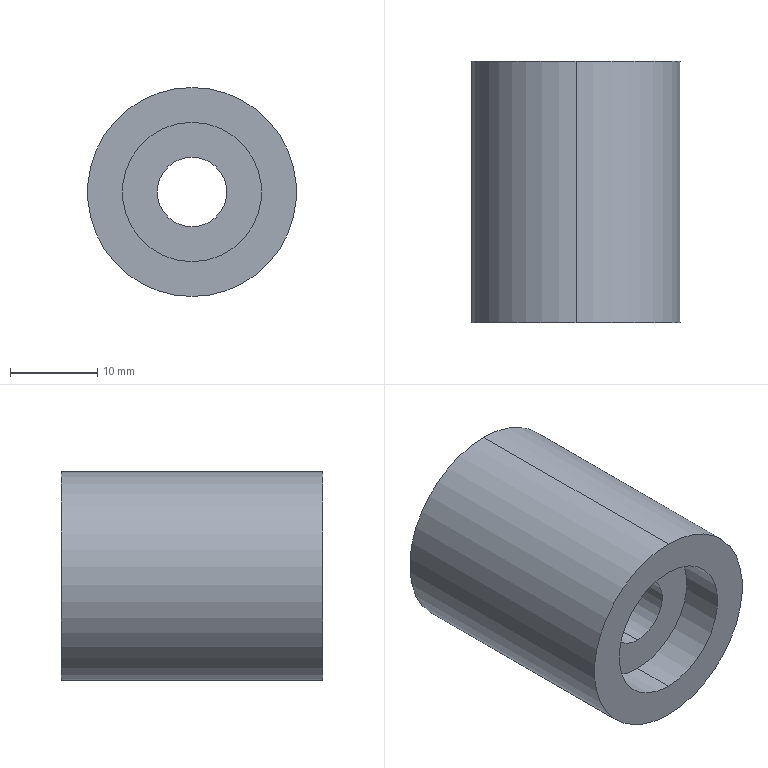Part | STEP file | Polisher small pulley | 1 solid | 12 faces | box 24 x 30 x 24 mm | volume 10556 mm3 | cylinder 8 | plane 4 | commonest cylinder face diameters 16 x4 8 x2 24 x2
STEP:
#1=CARTESIAN_POINT('',(0.,0.,0.));
#2=DIRECTION('',(0.,0.,1.));
#3=DIRECTION('',(1.,0.,0.));
#4=AXIS2_PLACEMENT_3D('',#1,#2,#3);
#5=CARTESIAN_POINT('',(0.,-10.,-8.));
#6=VERTEX_POINT('',#5);
#7=CARTESIAN_POINT('',(0.,-15.,-8.));
#8=VERTEX_POINT('',#7);
#9=CARTESIAN_POINT('',(0.,-10.,-8.));
#10=DIRECTION('',(0.,-1.,0.));
#11=VECTOR('',#10,1.);
#12=LINE('',#9,#11);
#13=CARTESIAN_POINT('',(0.,-10.,0.));
#14=DIRECTION('',(0.,-1.,0.));
#15=DIRECTION('',(0.,0.,-1.));
#16=AXIS2_PLACEMENT_3D('',#13,#14,#15);
#17=CYLINDRICAL_SURFACE('',#16,8.);
#18=CARTESIAN_POINT('',(6.283,0.));
#19=DIRECTION('',(0.,1.));
#20=VECTOR('',#19,1.);
#21=LINE('',#18,#20);
#22=(GEOMETRIC_REPRESENTATION_CONTEXT(2)PARAMETRIC_REPRESENTATION_CONTEXT()REPRESENTATION_CONTEXT('',''));
#23=DEFINITIONAL_REPRESENTATION('',(#21),#22);
#24=PCURVE('',#17,#23);
#25=CARTESIAN_POINT('',(0.,-10.,0.));
#26=DIRECTION('',(0.,-1.,0.));
#27=DIRECTION('',(0.,0.,-1.));
#28=AXIS2_PLACEMENT_3D('',#25,#26,#27);
#29=CYLINDRICAL_SURFACE('',#28,8.);
#30=CARTESIAN_POINT('',(0.,0.));
#31=DIRECTION('',(0.,1.));
#32=VECTOR('',#31,1.);
#33=LINE('',#30,#32);
#34=(GEOMETRIC_REPRESENTATION_CONTEXT(2)PARAMETRIC_REPRESENTATION_CONTEXT()REPRESENTATION_CONTEXT('',''));
#35=DEFINITIONAL_REPRESENTATION('',(#33),#34);
#36=PCURVE('',#29,#35);
#37=SURFACE_CURVE('',#12,(#24,#36),.PCURVE_S1.);
#38=EDGE_CURVE('',#6,#8,#37,.T.);
#39=ORIENTED_EDGE('',*,*,#38,.T.);
#40=CARTESIAN_POINT('',(0.,-15.,8.));
#41=VERTEX_POINT('',#40);
#42=CARTESIAN_POINT('',(0.,-15.,0.));
#43=DIRECTION('',(0.,-1.,0.));
#44=DIRECTION('',(0.,0.,-1.));
#45=AXIS2_PLACEMENT_3D('',#42,#43,#44);
#46=CIRCLE('',#45,8.);
#47=CARTESIAN_POINT('',(0.,5.));
#48=DIRECTION('',(1.,0.));
#49=VECTOR('',#48,1.);
#50=LINE('',#47,#49);
#51=(GEOMETRIC_REPRESENTATION_CONTEXT(2)PARAMETRIC_REPRESENTATION_CONTEXT()REPRESENTATION_CONTEXT('',''));
#52=DEFINITIONAL_REPRESENTATION('',(#50),#51);
#53=PCURVE('',#17,#52);
#54=CARTESIAN_POINT('',(0.,-15.,0.));
#55=DIRECTION('',(0.,1.,0.));
#56=DIRECTION('',(0.,0.,1.));
#57=AXIS2_PLACEMENT_3D('',#54,#55,#56);
#58=PLANE('',#57);
#59=CARTESIAN_POINT('',(-8.,0.));
#60=CARTESIAN_POINT('',(-8.,13.856));
#61=CARTESIAN_POINT('',(4.,6.928));
#62=CARTESIAN_POINT('',(16.,0.));
#63=CARTESIAN_POINT('',(4.,-6.928));
#64=CARTESIAN_POINT('',(-8.,-13.856));
#65=CARTESIAN_POINT('',(-8.,0.));
#66=(BOUNDED_CURVE()B_SPLINE_CURVE(2,(#59,#60,#61,#62,#63,#64,#65),.UNSPECIFIED.,.T.,.F.)B_SPLINE_CURVE_WITH_KNOTS((1,2,2,2,2,1),(-2.094,0.,2.094,4.189,6.283,8.378),.UNSPECIFIED.)CURVE()GEOMETRIC_REPRESENTATION_ITEM()RATIONAL_B_SPLINE_CURVE((1.,0.5,1.,0.5,1.,0.5,1.))REPRESENTATION_ITEM(''));
#67=(GEOMETRIC_REPRESENTATION_CONTEXT(2)PARAMETRIC_REPRESENTATION_CONTEXT()REPRESENTATION_CONTEXT('',''));
#68=DEFINITIONAL_REPRESENTATION('',(#66),#67);
#69=PCURVE('',#58,#68);
#70=SURFACE_CURVE('',#46,(#53,#69),.PCURVE_S1.);
#71=EDGE_CURVE('',#41,#8,#70,.T.);
#72=ORIENTED_EDGE('',*,*,#71,.F.);
#73=CARTESIAN_POINT('',(0.,-10.,8.));
#74=VERTEX_POINT('',#73);
#75=CARTESIAN_POINT('',(0.,-10.,8.));
#76=DIRECTION('',(0.,-1.,0.));
#77=VECTOR('',#76,1.);
#78=LINE('',#75,#77);
#79=CARTESIAN_POINT('',(3.142,0.));
#80=DIRECTION('',(0.,1.));
#81=VECTOR('',#80,1.);
#82=LINE('',#79,#81);
#83=(GEOMETRIC_REPRESENTATION_CONTEXT(2)PARAMETRIC_REPRESENTATION_CONTEXT()REPRESENTATION_CONTEXT('',''));
#84=DEFINITIONAL_REPRESENTATION('',(#82),#83);
#85=PCURVE('',#17,#84);
#86=CARTESIAN_POINT('',(3.142,0.));
#87=DIRECTION('',(0.,1.));
#88=VECTOR('',#87,1.);
#89=LINE('',#86,#88);
#90=(GEOMETRIC_REPRESENTATION_CONTEXT(2)PARAMETRIC_REPRESENTATION_CONTEXT()REPRESENTATION_CONTEXT('',''));
#91=DEFINITIONAL_REPRESENTATION('',(#89),#90);
#92=PCURVE('',#29,#91);
#93=SURFACE_CURVE('',#78,(#85,#92),.PCURVE_S1.);
#94=EDGE_CURVE('',#74,#41,#93,.T.);
#95=ORIENTED_EDGE('',*,*,#94,.F.);
#96=CARTESIAN_POINT('',(0.,-10.,0.));
#97=DIRECTION('',(0.,-1.,0.));
#98=DIRECTION('',(0.,0.,-1.));
#99=AXIS2_PLACEMENT_3D('',#96,#97,#98);
#100=CIRCLE('',#99,8.);
#101=CARTESIAN_POINT('',(0.,0.));
#102=DIRECTION('',(1.,0.));
#103=VECTOR('',#102,1.);
#104=LINE('',#101,#103);
#105=(GEOMETRIC_REPRESENTATION_CONTEXT(2)PARAMETRIC_REPRESENTATION_CONTEXT()REPRESENTATION_CONTEXT('',''));
#106=DEFINITIONAL_REPRESENTATION('',(#104),#105);
#107=PCURVE('',#17,#106);
#108=CARTESIAN_POINT('',(0.,-10.,0.));
#109=DIRECTION('',(0.,-1.,0.));
#110=DIRECTION('',(0.,0.,-1.));
#111=AXIS2_PLACEMENT_3D('',#108,#109,#110);
#112=PLANE('',#111);
#113=CARTESIAN_POINT('',(0.,0.));
#114=DIRECTION('',(1.,0.));
#115=AXIS2_PLACEMENT_2D('',#113,#114);
#116=CIRCLE('',#115,8.);
#117=(GEOMETRIC_REPRESENTATION_CONTEXT(2)PARAMETRIC_REPRESENTATION_CONTEXT()REPRESENTATION_CONTEXT('',''));
#118=DEFINITIONAL_REPRESENTATION('',(#116),#117);
#119=PCURVE('',#112,#118);
#120=SURFACE_CURVE('',#100,(#107,#119),.PCURVE_S1.);
#121=EDGE_CURVE('',#74,#6,#120,.T.);
#122=ORIENTED_EDGE('',*,*,#121,.T.);
#123=EDGE_LOOP('',(#39,#72,#95,#122));
#124=FACE_BOUND('',#123,.F.);
#125=ADVANCED_FACE('',(#124),#17,.F.);
#126=CARTESIAN_POINT('',(0.,10.,8.));
#127=VERTEX_POINT('',#126);
#128=CARTESIAN_POINT('',(0.,15.,8.));
#129=VERTEX_POINT('',#128);
#130=CARTESIAN_POINT('',(0.,10.,8.));
#131=DIRECTION('',(0.,1.,0.));
#132=VECTOR('',#131,1.);
#133=LINE('',#130,#132);
#134=CARTESIAN_POINT('',(0.,10.,0.));
#135=DIRECTION('',(0.,1.,0.));
#136=DIRECTION('',(0.,0.,1.));
#137=AXIS2_PLACEMENT_3D('',#134,#135,#136);
#138=CYLINDRICAL_SURFACE('',#137,8.);
#139=CARTESIAN_POINT('',(6.283,0.));
#140=DIRECTION('',(0.,1.));
#141=VECTOR('',#140,1.);
#142=LINE('',#139,#141);
#143=(GEOMETRIC_REPRESENTATION_CONTEXT(2)PARAMETRIC_REPRESENTATION_CONTEXT()REPRESENTATION_CONTEXT('',''));
#144=DEFINITIONAL_REPRESENTATION('',(#142),#143);
#145=PCURVE('',#138,#144);
#146=CARTESIAN_POINT('',(0.,10.,0.));
#147=DIRECTION('',(0.,1.,0.));
#148=DIRECTION('',(0.,0.,1.));
#149=AXIS2_PLACEMENT_3D('',#146,#147,#148);
#150=CYLINDRICAL_SURFACE('',#149,8.);
#151=CARTESIAN_POINT('',(0.,0.));
#152=DIRECTION('',(0.,1.));
#153=VECTOR('',#152,1.);
#154=LINE('',#151,#153);
#155=(GEOMETRIC_REPRESENTATION_CONTEXT(2)PARAMETRIC_REPRESENTATION_CONTEXT()REPRESENTATION_CONTEXT('',''));
#156=DEFINITIONAL_REPRESENTATION('',(#154),#155);
#157=PCURVE('',#150,#156);
#158=SURFACE_CURVE('',#133,(#145,#157),.PCURVE_S1.);
#159=EDGE_CURVE('',#127,#129,#158,.T.);
#160=ORIENTED_EDGE('',*,*,#159,.T.);
#161=CARTESIAN_POINT('',(0.,15.,-8.));
#162=VERTEX_POINT('',#161);
#163=CARTESIAN_POINT('',(0.,15.,0.));
#164=DIRECTION('',(0.,1.,0.));
#165=DIRECTION('',(0.,0.,1.));
#166=AXIS2_PLACEMENT_3D('',#163,#164,#165);
#167=CIRCLE('',#166,8.);
#168=CARTESIAN_POINT('',(0.,5.));
#169=DIRECTION('',(1.,0.));
#170=VECTOR('',#169,1.);
#171=LINE('',#168,#170);
#172=(GEOMETRIC_REPRESENTATION_CONTEXT(2)PARAMETRIC_REPRESENTATION_CONTEXT()REPRESENTATION_CONTEXT('',''));
#173=DEFINITIONAL_REPRESENTATION('',(#171),#172);
#174=PCURVE('',#138,#173);
#175=CARTESIAN_POINT('',(0.,15.,0.));
#176=DIRECTION('',(0.,1.,0.));
#177=DIRECTION('',(0.,0.,1.));
#178=AXIS2_PLACEMENT_3D('',#175,#176,#177);
#179=PLANE('',#178);
#180=CARTESIAN_POINT('',(0.,0.));
#181=DIRECTION('',(1.,0.));
#182=AXIS2_PLACEMENT_2D('',#180,#181);
#183=CIRCLE('',#182,8.);
#184=(GEOMETRIC_REPRESENTATION_CONTEXT(2)PARAMETRIC_REPRESENTATION_CONTEXT()REPRESENTATION_CONTEXT('',''));
#185=DEFINITIONAL_REPRESENTATION('',(#183),#184);
#186=PCURVE('',#179,#185);
#187=SURFACE_CURVE('',#167,(#174,#186),.PCURVE_S1.);
#188=EDGE_CURVE('',#162,#129,#187,.T.);
#189=ORIENTED_EDGE('',*,*,#188,.F.);
#190=CARTESIAN_POINT('',(0.,10.,-8.));
#191=VERTEX_POINT('',#190);
#192=CARTESIAN_POINT('',(0.,10.,-8.));
#193=DIRECTION('',(0.,1.,0.));
#194=VECTOR('',#193,1.);
#195=LINE('',#192,#194);
#196=CARTESIAN_POINT('',(3.142,0.));
#197=DIRECTION('',(0.,1.));
#198=VECTOR('',#197,1.);
#199=LINE('',#196,#198);
#200=(GEOMETRIC_REPRESENTATION_CONTEXT(2)PARAMETRIC_REPRESENTATION_CONTEXT()REPRESENTATION_CONTEXT('',''));
#201=DEFINITIONAL_REPRESENTATION('',(#199),#200);
#202=PCURVE('',#138,#201);
#203=CARTESIAN_POINT('',(3.142,0.));
#204=DIRECTION('',(0.,1.));
#205=VECTOR('',#204,1.);
#206=LINE('',#203,#205);
#207=(GEOMETRIC_REPRESENTATION_CONTEXT(2)PARAMETRIC_REPRESENTATION_CONTEXT()REPRESENTATION_CONTEXT('',''));
#208=DEFINITIONAL_REPRESENTATION('',(#206),#207);
#209=PCURVE('',#150,#208);
#210=SURFACE_CURVE('',#195,(#202,#209),.PCURVE_S1.);
#211=EDGE_CURVE('',#191,#162,#210,.T.);
#212=ORIENTED_EDGE('',*,*,#211,.F.);
#213=CARTESIAN_POINT('',(0.,10.,0.));
#214=DIRECTION('',(0.,1.,0.));
#215=DIRECTION('',(0.,0.,1.));
#216=AXIS2_PLACEMENT_3D('',#213,#214,#215);
#217=CIRCLE('',#216,8.);
#218=CARTESIAN_POINT('',(0.,0.));
#219=DIRECTION('',(1.,0.));
#220=VECTOR('',#219,1.);
#221=LINE('',#218,#220);
#222=(GEOMETRIC_REPRESENTATION_CONTEXT(2)PARAMETRIC_REPRESENTATION_CONTEXT()REPRESENTATION_CONTEXT('',''));
#223=DEFINITIONAL_REPRESENTATION('',(#221),#222);
#224=PCURVE('',#138,#223);
#225=CARTESIAN_POINT('',(0.,10.,0.));
#226=DIRECTION('',(0.,1.,0.));
#227=DIRECTION('',(0.,0.,1.));
#228=AXIS2_PLACEMENT_3D('',#225,#226,#227);
#229=PLANE('',#228);
#230=CARTESIAN_POINT('',(0.,0.));
#231=DIRECTION('',(1.,0.));
#232=AXIS2_PLACEMENT_2D('',#230,#231);
#233=CIRCLE('',#232,8.);
#234=(GEOMETRIC_REPRESENTATION_CONTEXT(2)PARAMETRIC_REPRESENTATION_CONTEXT()REPRESENTATION_CONTEXT('',''));
#235=DEFINITIONAL_REPRESENTATION('',(#233),#234);
#236=PCURVE('',#229,#235);
#237=SURFACE_CURVE('',#217,(#224,#236),.PCURVE_S1.);
#238=EDGE_CURVE('',#191,#127,#237,.T.);
#239=ORIENTED_EDGE('',*,*,#238,.T.);
#240=EDGE_LOOP('',(#160,#189,#212,#239));
#241=FACE_BOUND('',#240,.F.);
#242=ADVANCED_FACE('',(#241),#138,.F.);
#243=CARTESIAN_POINT('',(0.,15.,12.));
#244=VERTEX_POINT('',#243);
#245=CARTESIAN_POINT('',(0.,15.,-12.));
#246=VERTEX_POINT('',#245);
#247=CARTESIAN_POINT('',(0.,15.,0.));
#248=DIRECTION('',(0.,1.,0.));
#249=DIRECTION('',(0.,0.,1.));
#250=AXIS2_PLACEMENT_3D('',#247,#248,#249);
#251=CIRCLE('',#250,12.);
#252=CARTESIAN_POINT('',(0.,15.,0.));
#253=DIRECTION('',(0.,-1.,0.));
#254=DIRECTION('',(0.,0.,-1.));
#255=AXIS2_PLACEMENT_3D('',#252,#253,#254);
#256=CYLINDRICAL_SURFACE('',#255,12.);
#257=CARTESIAN_POINT('',(3.142,0.));
#258=DIRECTION('',(-1.,0.));
#259=VECTOR('',#258,1.);
#260=LINE('',#257,#259);
#261=(GEOMETRIC_REPRESENTATION_CONTEXT(2)PARAMETRIC_REPRESENTATION_CONTEXT()REPRESENTATION_CONTEXT('',''));
#262=DEFINITIONAL_REPRESENTATION('',(#260),#261);
#263=PCURVE('',#256,#262);
#264=CARTESIAN_POINT('',(0.,0.));
#265=DIRECTION('',(1.,0.));
#266=AXIS2_PLACEMENT_2D('',#264,#265);
#267=CIRCLE('',#266,12.);
#268=(GEOMETRIC_REPRESENTATION_CONTEXT(2)PARAMETRIC_REPRESENTATION_CONTEXT()REPRESENTATION_CONTEXT('',''));
#269=DEFINITIONAL_REPRESENTATION('',(#267),#268);
#270=PCURVE('',#179,#269);
#271=SURFACE_CURVE('',#251,(#263,#270),.PCURVE_S1.);
#272=EDGE_CURVE('',#244,#246,#271,.T.);
#273=ORIENTED_EDGE('',*,*,#272,.F.);
#274=CARTESIAN_POINT('',(0.,-15.,12.));
#275=VERTEX_POINT('',#274);
#276=CARTESIAN_POINT('',(0.,15.,12.));
#277=DIRECTION('',(0.,-1.,0.));
#278=VECTOR('',#277,1.);
#279=LINE('',#276,#278);
#280=CARTESIAN_POINT('',(3.142,0.));
#281=DIRECTION('',(0.,1.));
#282=VECTOR('',#281,1.);
#283=LINE('',#280,#282);
#284=(GEOMETRIC_REPRESENTATION_CONTEXT(2)PARAMETRIC_REPRESENTATION_CONTEXT()REPRESENTATION_CONTEXT('',''));
#285=DEFINITIONAL_REPRESENTATION('',(#283),#284);
#286=PCURVE('',#256,#285);
#287=CARTESIAN_POINT('',(0.,15.,0.));
#288=DIRECTION('',(0.,-1.,0.));
#289=DIRECTION('',(0.,0.,-1.));
#290=AXIS2_PLACEMENT_3D('',#287,#288,#289);
#291=CYLINDRICAL_SURFACE('',#290,12.);
#292=CARTESIAN_POINT('',(3.142,0.));
#293=DIRECTION('',(0.,1.));
#294=VECTOR('',#293,1.);
#295=LINE('',#292,#294);
#296=(GEOMETRIC_REPRESENTATION_CONTEXT(2)PARAMETRIC_REPRESENTATION_CONTEXT()REPRESENTATION_CONTEXT('',''));
#297=DEFINITIONAL_REPRESENTATION('',(#295),#296);
#298=PCURVE('',#291,#297);
#299=SURFACE_CURVE('',#279,(#286,#298),.PCURVE_S1.);
#300=EDGE_CURVE('',#244,#275,#299,.T.);
#301=ORIENTED_EDGE('',*,*,#300,.T.);
#302=CARTESIAN_POINT('',(0.,-15.,-12.));
#303=VERTEX_POINT('',#302);
#304=CARTESIAN_POINT('',(0.,-15.,0.));
#305=DIRECTION('',(0.,1.,0.));
#306=DIRECTION('',(0.,0.,1.));
#307=AXIS2_PLACEMENT_3D('',#304,#305,#306);
#308=CIRCLE('',#307,12.);
#309=CARTESIAN_POINT('',(3.142,30.));
#310=DIRECTION('',(-1.,0.));
#311=VECTOR('',#310,1.);
#312=LINE('',#309,#311);
#313=(GEOMETRIC_REPRESENTATION_CONTEXT(2)PARAMETRIC_REPRESENTATION_CONTEXT()REPRESENTATION_CONTEXT('',''));
#314=DEFINITIONAL_REPRESENTATION('',(#312),#313);
#315=PCURVE('',#256,#314);
#316=CARTESIAN_POINT('',(0.,0.));
#317=DIRECTION('',(1.,0.));
#318=AXIS2_PLACEMENT_2D('',#316,#317);
#319=CIRCLE('',#318,12.);
#320=(GEOMETRIC_REPRESENTATION_CONTEXT(2)PARAMETRIC_REPRESENTATION_CONTEXT()REPRESENTATION_CONTEXT('',''));
#321=DEFINITIONAL_REPRESENTATION('',(#319),#320);
#322=PCURVE('',#58,#321);
#323=SURFACE_CURVE('',#308,(#315,#322),.PCURVE_S1.);
#324=EDGE_CURVE('',#275,#303,#323,.T.);
#325=ORIENTED_EDGE('',*,*,#324,.T.);
#326=CARTESIAN_POINT('',(0.,15.,-12.));
#327=DIRECTION('',(0.,-1.,0.));
#328=VECTOR('',#327,1.);
#329=LINE('',#326,#328);
#330=CARTESIAN_POINT('',(0.,0.));
#331=DIRECTION('',(0.,1.));
#332=VECTOR('',#331,1.);
#333=LINE('',#330,#332);
#334=(GEOMETRIC_REPRESENTATION_CONTEXT(2)PARAMETRIC_REPRESENTATION_CONTEXT()REPRESENTATION_CONTEXT('',''));
#335=DEFINITIONAL_REPRESENTATION('',(#333),#334);
#336=PCURVE('',#256,#335);
#337=CARTESIAN_POINT('',(6.283,0.));
#338=DIRECTION('',(0.,1.));
#339=VECTOR('',#338,1.);
#340=LINE('',#337,#339);
#341=(GEOMETRIC_REPRESENTATION_CONTEXT(2)PARAMETRIC_REPRESENTATION_CONTEXT()REPRESENTATION_CONTEXT('',''));
#342=DEFINITIONAL_REPRESENTATION('',(#340),#341);
#343=PCURVE('',#291,#342);
#344=SURFACE_CURVE('',#329,(#336,#343),.PCURVE_S1.);
#345=EDGE_CURVE('',#246,#303,#344,.T.);
#346=ORIENTED_EDGE('',*,*,#345,.F.);
#347=EDGE_LOOP('',(#273,#301,#325,#346));
#348=FACE_BOUND('',#347,.T.);
#349=ADVANCED_FACE('',(#348),#256,.T.);
#350=CARTESIAN_POINT('',(0.,-10.,4.));
#351=VERTEX_POINT('',#350);
#352=CARTESIAN_POINT('',(0.,10.,4.));
#353=VERTEX_POINT('',#352);
#354=CARTESIAN_POINT('',(0.,-15.,4.));
#355=DIRECTION('',(0.,1.,0.));
#356=VECTOR('',#355,1.);
#357=LINE('',#354,#356);
#358=CARTESIAN_POINT('',(0.,-15.,0.));
#359=DIRECTION('',(0.,1.,0.));
#360=DIRECTION('',(0.,0.,1.));
#361=AXIS2_PLACEMENT_3D('',#358,#359,#360);
#362=CYLINDRICAL_SURFACE('',#361,4.);
#363=CARTESIAN_POINT('',(6.283,0.));
#364=DIRECTION('',(0.,1.));
#365=VECTOR('',#364,1.);
#366=LINE('',#363,#365);
#367=(GEOMETRIC_REPRESENTATION_CONTEXT(2)PARAMETRIC_REPRESENTATION_CONTEXT()REPRESENTATION_CONTEXT('',''));
#368=DEFINITIONAL_REPRESENTATION('',(#366),#367);
#369=PCURVE('',#362,#368);
#370=CARTESIAN_POINT('',(0.,-15.,0.));
#371=DIRECTION('',(0.,1.,0.));
#372=DIRECTION('',(0.,0.,1.));
#373=AXIS2_PLACEMENT_3D('',#370,#371,#372);
#374=CYLINDRICAL_SURFACE('',#373,4.);
#375=CARTESIAN_POINT('',(0.,0.));
#376=DIRECTION('',(0.,1.));
#377=VECTOR('',#376,1.);
#378=LINE('',#375,#377);
#379=(GEOMETRIC_REPRESENTATION_CONTEXT(2)PARAMETRIC_REPRESENTATION_CONTEXT()REPRESENTATION_CONTEXT('',''));
#380=DEFINITIONAL_REPRESENTATION('',(#378),#379);
#381=PCURVE('',#374,#380);
#382=SURFACE_CURVE('',#357,(#369,#381),.PCURVE_S1.);
#383=EDGE_CURVE('',#351,#353,#382,.T.);
#384=ORIENTED_EDGE('',*,*,#383,.T.);
#385=CARTESIAN_POINT('',(0.,10.,-4.));
#386=VERTEX_POINT('',#385);
#387=CARTESIAN_POINT('',(0.,10.,0.));
#388=DIRECTION('',(0.,1.,0.));
#389=DIRECTION('',(0.,0.,1.));
#390=AXIS2_PLACEMENT_3D('',#387,#388,#389);
#391=CIRCLE('',#390,4.);
#392=CARTESIAN_POINT('',(0.,25.));
#393=DIRECTION('',(1.,0.));
#394=VECTOR('',#393,1.);
#395=LINE('',#392,#394);
#396=(GEOMETRIC_REPRESENTATION_CONTEXT(2)PARAMETRIC_REPRESENTATION_CONTEXT()REPRESENTATION_CONTEXT('',''));
#397=DEFINITIONAL_REPRESENTATION('',(#395),#396);
#398=PCURVE('',#362,#397);
#399=CARTESIAN_POINT('',(0.,0.));
#400=DIRECTION('',(1.,0.));
#401=AXIS2_PLACEMENT_2D('',#399,#400);
#402=CIRCLE('',#401,4.);
#403=(GEOMETRIC_REPRESENTATION_CONTEXT(2)PARAMETRIC_REPRESENTATION_CONTEXT()REPRESENTATION_CONTEXT('',''));
#404=DEFINITIONAL_REPRESENTATION('',(#402),#403);
#405=PCURVE('',#229,#404);
#406=SURFACE_CURVE('',#391,(#398,#405),.PCURVE_S1.);
#407=EDGE_CURVE('',#386,#353,#406,.T.);
#408=ORIENTED_EDGE('',*,*,#407,.F.);
#409=CARTESIAN_POINT('',(0.,-10.,-4.));
#410=VERTEX_POINT('',#409);
#411=CARTESIAN_POINT('',(0.,-15.,-4.));
#412=DIRECTION('',(0.,1.,0.));
#413=VECTOR('',#412,1.);
#414=LINE('',#411,#413);
#415=CARTESIAN_POINT('',(3.142,0.));
#416=DIRECTION('',(0.,1.));
#417=VECTOR('',#416,1.);
#418=LINE('',#415,#417);
#419=(GEOMETRIC_REPRESENTATION_CONTEXT(2)PARAMETRIC_REPRESENTATION_CONTEXT()REPRESENTATION_CONTEXT('',''));
#420=DEFINITIONAL_REPRESENTATION('',(#418),#419);
#421=PCURVE('',#362,#420);
#422=CARTESIAN_POINT('',(3.142,0.));
#423=DIRECTION('',(0.,1.));
#424=VECTOR('',#423,1.);
#425=LINE('',#422,#424);
#426=(GEOMETRIC_REPRESENTATION_CONTEXT(2)PARAMETRIC_REPRESENTATION_CONTEXT()REPRESENTATION_CONTEXT('',''));
#427=DEFINITIONAL_REPRESENTATION('',(#425),#426);
#428=PCURVE('',#374,#427);
#429=SURFACE_CURVE('',#414,(#421,#428),.PCURVE_S1.);
#430=EDGE_CURVE('',#410,#386,#429,.T.);
#431=ORIENTED_EDGE('',*,*,#430,.F.);
#432=CARTESIAN_POINT('',(0.,-10.,0.));
#433=DIRECTION('',(0.,1.,0.));
#434=DIRECTION('',(0.,0.,-1.));
#435=AXIS2_PLACEMENT_3D('',#432,#433,#434);
#436=CIRCLE('',#435,4.);
#437=CARTESIAN_POINT('',(3.142,5.));
#438=DIRECTION('',(1.,0.));
#439=VECTOR('',#438,1.);
#440=LINE('',#437,#439);
#441=(GEOMETRIC_REPRESENTATION_CONTEXT(2)PARAMETRIC_REPRESENTATION_CONTEXT()REPRESENTATION_CONTEXT('',''));
#442=DEFINITIONAL_REPRESENTATION('',(#440),#441);
#443=PCURVE('',#362,#442);
#444=CARTESIAN_POINT('',(4.,0.));
#445=CARTESIAN_POINT('',(4.,-6.928));
#446=CARTESIAN_POINT('',(-2.,-3.464));
#447=CARTESIAN_POINT('',(-8.,0.));
#448=CARTESIAN_POINT('',(-2.,3.464));
#449=CARTESIAN_POINT('',(4.,6.928));
#450=CARTESIAN_POINT('',(4.,0.));
#451=(BOUNDED_CURVE()B_SPLINE_CURVE(2,(#444,#445,#446,#447,#448,#449,#450),.UNSPECIFIED.,.T.,.F.)B_SPLINE_CURVE_WITH_KNOTS((1,2,2,2,2,1),(-2.094,0.,2.094,4.189,6.283,8.378),.UNSPECIFIED.)CURVE()GEOMETRIC_REPRESENTATION_ITEM()RATIONAL_B_SPLINE_CURVE((1.,0.5,1.,0.5,1.,0.5,1.))REPRESENTATION_ITEM(''));
#452=(GEOMETRIC_REPRESENTATION_CONTEXT(2)PARAMETRIC_REPRESENTATION_CONTEXT()REPRESENTATION_CONTEXT('',''));
#453=DEFINITIONAL_REPRESENTATION('',(#451),#452);
#454=PCURVE('',#112,#453);
#455=SURFACE_CURVE('',#436,(#443,#454),.PCURVE_S1.);
#456=EDGE_CURVE('',#410,#351,#455,.T.);
#457=ORIENTED_EDGE('',*,*,#456,.T.);
#458=EDGE_LOOP('',(#384,#408,#431,#457));
#459=FACE_BOUND('',#458,.F.);
#460=ADVANCED_FACE('',(#459),#362,.F.);
#461=CARTESIAN_POINT('',(0.,10.,0.));
#462=DIRECTION('',(0.,1.,0.));
#463=DIRECTION('',(0.,0.,1.));
#464=AXIS2_PLACEMENT_3D('',#461,#462,#463);
#465=CIRCLE('',#464,4.);
#466=CARTESIAN_POINT('',(0.,25.));
#467=DIRECTION('',(1.,0.));
#468=VECTOR('',#467,1.);
#469=LINE('',#466,#468);
#470=(GEOMETRIC_REPRESENTATION_CONTEXT(2)PARAMETRIC_REPRESENTATION_CONTEXT()REPRESENTATION_CONTEXT('',''));
#471=DEFINITIONAL_REPRESENTATION('',(#469),#470);
#472=PCURVE('',#374,#471);
#473=CARTESIAN_POINT('',(0.,0.));
#474=DIRECTION('',(1.,0.));
#475=AXIS2_PLACEMENT_2D('',#473,#474);
#476=CIRCLE('',#475,4.);
#477=(GEOMETRIC_REPRESENTATION_CONTEXT(2)PARAMETRIC_REPRESENTATION_CONTEXT()REPRESENTATION_CONTEXT('',''));
#478=DEFINITIONAL_REPRESENTATION('',(#476),#477);
#479=PCURVE('',#229,#478);
#480=SURFACE_CURVE('',#465,(#472,#479),.PCURVE_S1.);
#481=EDGE_CURVE('',#353,#386,#480,.T.);
#482=ORIENTED_EDGE('',*,*,#481,.F.);
#483=ORIENTED_EDGE('',*,*,#383,.F.);
#484=CARTESIAN_POINT('',(0.,-10.,0.));
#485=DIRECTION('',(0.,1.,0.));
#486=DIRECTION('',(0.,0.,-1.));
#487=AXIS2_PLACEMENT_3D('',#484,#485,#486);
#488=CIRCLE('',#487,4.);
#489=CARTESIAN_POINT('',(-3.142,5.));
#490=DIRECTION('',(1.,0.));
#491=VECTOR('',#490,1.);
#492=LINE('',#489,#491);
#493=(GEOMETRIC_REPRESENTATION_CONTEXT(2)PARAMETRIC_REPRESENTATION_CONTEXT()REPRESENTATION_CONTEXT('',''));
#494=DEFINITIONAL_REPRESENTATION('',(#492),#493);
#495=PCURVE('',#374,#494);
#496=CARTESIAN_POINT('',(4.,0.));
#497=CARTESIAN_POINT('',(4.,-6.928));
#498=CARTESIAN_POINT('',(-2.,-3.464));
#499=CARTESIAN_POINT('',(-8.,0.));
#500=CARTESIAN_POINT('',(-2.,3.464));
#501=CARTESIAN_POINT('',(4.,6.928));
#502=CARTESIAN_POINT('',(4.,0.));
#503=(BOUNDED_CURVE()B_SPLINE_CURVE(2,(#496,#497,#498,#499,#500,#501,#502),.UNSPECIFIED.,.T.,.F.)B_SPLINE_CURVE_WITH_KNOTS((1,2,2,2,2,1),(-2.094,0.,2.094,4.189,6.283,8.378),.UNSPECIFIED.)CURVE()GEOMETRIC_REPRESENTATION_ITEM()RATIONAL_B_SPLINE_CURVE((1.,0.5,1.,0.5,1.,0.5,1.))REPRESENTATION_ITEM(''));
#504=(GEOMETRIC_REPRESENTATION_CONTEXT(2)PARAMETRIC_REPRESENTATION_CONTEXT()REPRESENTATION_CONTEXT('',''));
#505=DEFINITIONAL_REPRESENTATION('',(#503),#504);
#506=PCURVE('',#112,#505);
#507=SURFACE_CURVE('',#488,(#495,#506),.PCURVE_S1.);
#508=EDGE_CURVE('',#351,#410,#507,.T.);
#509=ORIENTED_EDGE('',*,*,#508,.T.);
#510=ORIENTED_EDGE('',*,*,#430,.T.);
#511=EDGE_LOOP('',(#482,#483,#509,#510));
#512=FACE_BOUND('',#511,.F.);
#513=ADVANCED_FACE('',(#512),#374,.F.);
#514=ORIENTED_EDGE('',*,*,#300,.F.);
#515=CARTESIAN_POINT('',(0.,15.,0.));
#516=DIRECTION('',(0.,1.,0.));
#517=DIRECTION('',(0.,0.,1.));
#518=AXIS2_PLACEMENT_3D('',#515,#516,#517);
#519=CIRCLE('',#518,12.);
#520=CARTESIAN_POINT('',(9.425,0.));
#521=DIRECTION('',(-1.,0.));
#522=VECTOR('',#521,1.);
#523=LINE('',#520,#522);
#524=(GEOMETRIC_REPRESENTATION_CONTEXT(2)PARAMETRIC_REPRESENTATION_CONTEXT()REPRESENTATION_CONTEXT('',''));
#525=DEFINITIONAL_REPRESENTATION('',(#523),#524);
#526=PCURVE('',#291,#525);
#527=CARTESIAN_POINT('',(0.,0.));
#528=DIRECTION('',(1.,0.));
#529=AXIS2_PLACEMENT_2D('',#527,#528);
#530=CIRCLE('',#529,12.);
#531=(GEOMETRIC_REPRESENTATION_CONTEXT(2)PARAMETRIC_REPRESENTATION_CONTEXT()REPRESENTATION_CONTEXT('',''));
#532=DEFINITIONAL_REPRESENTATION('',(#530),#531);
#533=PCURVE('',#179,#532);
#534=SURFACE_CURVE('',#519,(#526,#533),.PCURVE_S1.);
#535=EDGE_CURVE('',#246,#244,#534,.T.);
#536=ORIENTED_EDGE('',*,*,#535,.F.);
#537=ORIENTED_EDGE('',*,*,#345,.T.);
#538=CARTESIAN_POINT('',(0.,-15.,0.));
#539=DIRECTION('',(0.,1.,0.));
#540=DIRECTION('',(0.,0.,1.));
#541=AXIS2_PLACEMENT_3D('',#538,#539,#540);
#542=CIRCLE('',#541,12.);
#543=CARTESIAN_POINT('',(9.425,30.));
#544=DIRECTION('',(-1.,0.));
#545=VECTOR('',#544,1.);
#546=LINE('',#543,#545);
#547=(GEOMETRIC_REPRESENTATION_CONTEXT(2)PARAMETRIC_REPRESENTATION_CONTEXT()REPRESENTATION_CONTEXT('',''));
#548=DEFINITIONAL_REPRESENTATION('',(#546),#547);
#549=PCURVE('',#291,#548);
#550=CARTESIAN_POINT('',(0.,0.));
#551=DIRECTION('',(1.,0.));
#552=AXIS2_PLACEMENT_2D('',#550,#551);
#553=CIRCLE('',#552,12.);
#554=(GEOMETRIC_REPRESENTATION_CONTEXT(2)PARAMETRIC_REPRESENTATION_CONTEXT()REPRESENTATION_CONTEXT('',''));
#555=DEFINITIONAL_REPRESENTATION('',(#553),#554);
#556=PCURVE('',#58,#555);
#557=SURFACE_CURVE('',#542,(#549,#556),.PCURVE_S1.);
#558=EDGE_CURVE('',#303,#275,#557,.T.);
#559=ORIENTED_EDGE('',*,*,#558,.T.);
#560=EDGE_LOOP('',(#514,#536,#537,#559));
#561=FACE_BOUND('',#560,.T.);
#562=ADVANCED_FACE('',(#561),#291,.T.);
#563=CARTESIAN_POINT('',(0.,15.,0.));
#564=DIRECTION('',(0.,1.,0.));
#565=DIRECTION('',(0.,0.,1.));
#566=AXIS2_PLACEMENT_3D('',#563,#564,#565);
#567=CIRCLE('',#566,8.);
#568=CARTESIAN_POINT('',(0.,0.));
#569=DIRECTION('',(1.,0.));
#570=AXIS2_PLACEMENT_2D('',#568,#569);
#571=CIRCLE('',#570,8.);
#572=(GEOMETRIC_REPRESENTATION_CONTEXT(2)PARAMETRIC_REPRESENTATION_CONTEXT()REPRESENTATION_CONTEXT('',''));
#573=DEFINITIONAL_REPRESENTATION('',(#571),#572);
#574=PCURVE('',#179,#573);
#575=CARTESIAN_POINT('',(0.,5.));
#576=DIRECTION('',(1.,0.));
#577=VECTOR('',#576,1.);
#578=LINE('',#575,#577);
#579=(GEOMETRIC_REPRESENTATION_CONTEXT(2)PARAMETRIC_REPRESENTATION_CONTEXT()REPRESENTATION_CONTEXT('',''));
#580=DEFINITIONAL_REPRESENTATION('',(#578),#579);
#581=PCURVE('',#150,#580);
#582=SURFACE_CURVE('',#567,(#574,#581),.PCURVE_S1.);
#583=EDGE_CURVE('',#129,#162,#582,.T.);
#584=ORIENTED_EDGE('',*,*,#583,.F.);
#585=ORIENTED_EDGE('',*,*,#188,.F.);
#586=EDGE_LOOP('',(#584,#585));
#587=FACE_BOUND('',#586,.T.);
#588=ORIENTED_EDGE('',*,*,#535,.T.);
#589=ORIENTED_EDGE('',*,*,#272,.T.);
#590=EDGE_LOOP('',(#588,#589));
#591=FACE_BOUND('',#590,.T.);
#592=ADVANCED_FACE('',(#587,#591),#179,.T.);
#593=CARTESIAN_POINT('',(0.,-15.,0.));
#594=DIRECTION('',(0.,-1.,0.));
#595=DIRECTION('',(0.,0.,-1.));
#596=AXIS2_PLACEMENT_3D('',#593,#594,#595);
#597=CIRCLE('',#596,8.);
#598=CARTESIAN_POINT('',(-8.,0.));
#599=CARTESIAN_POINT('',(-8.,13.856));
#600=CARTESIAN_POINT('',(4.,6.928));
#601=CARTESIAN_POINT('',(16.,0.));
#602=CARTESIAN_POINT('',(4.,-6.928));
#603=CARTESIAN_POINT('',(-8.,-13.856));
#604=CARTESIAN_POINT('',(-8.,0.));
#605=(BOUNDED_CURVE()B_SPLINE_CURVE(2,(#598,#599,#600,#601,#602,#603,#604),.UNSPECIFIED.,.T.,.F.)B_SPLINE_CURVE_WITH_KNOTS((1,2,2,2,2,1),(-2.094,0.,2.094,4.189,6.283,8.378),.UNSPECIFIED.)CURVE()GEOMETRIC_REPRESENTATION_ITEM()RATIONAL_B_SPLINE_CURVE((1.,0.5,1.,0.5,1.,0.5,1.))REPRESENTATION_ITEM(''));
#606=(GEOMETRIC_REPRESENTATION_CONTEXT(2)PARAMETRIC_REPRESENTATION_CONTEXT()REPRESENTATION_CONTEXT('',''));
#607=DEFINITIONAL_REPRESENTATION('',(#605),#606);
#608=PCURVE('',#58,#607);
#609=CARTESIAN_POINT('',(0.,5.));
#610=DIRECTION('',(1.,0.));
#611=VECTOR('',#610,1.);
#612=LINE('',#609,#611);
#613=(GEOMETRIC_REPRESENTATION_CONTEXT(2)PARAMETRIC_REPRESENTATION_CONTEXT()REPRESENTATION_CONTEXT('',''));
#614=DEFINITIONAL_REPRESENTATION('',(#612),#613);
#615=PCURVE('',#29,#614);
#616=SURFACE_CURVE('',#597,(#608,#615),.PCURVE_S1.);
#617=EDGE_CURVE('',#8,#41,#616,.T.);
#618=ORIENTED_EDGE('',*,*,#617,.F.);
#619=ORIENTED_EDGE('',*,*,#71,.F.);
#620=EDGE_LOOP('',(#618,#619));
#621=FACE_BOUND('',#620,.T.);
#622=ORIENTED_EDGE('',*,*,#558,.F.);
#623=ORIENTED_EDGE('',*,*,#324,.F.);
#624=EDGE_LOOP('',(#622,#623));
#625=FACE_BOUND('',#624,.T.);
#626=ADVANCED_FACE('',(#621,#625),#58,.F.);
#627=ORIENTED_EDGE('',*,*,#583,.F.);
#628=ORIENTED_EDGE('',*,*,#159,.F.);
#629=CARTESIAN_POINT('',(0.,10.,0.));
#630=DIRECTION('',(0.,1.,0.));
#631=DIRECTION('',(0.,0.,1.));
#632=AXIS2_PLACEMENT_3D('',#629,#630,#631);
#633=CIRCLE('',#632,8.);
#634=CARTESIAN_POINT('',(0.,0.));
#635=DIRECTION('',(1.,0.));
#636=VECTOR('',#635,1.);
#637=LINE('',#634,#636);
#638=(GEOMETRIC_REPRESENTATION_CONTEXT(2)PARAMETRIC_REPRESENTATION_CONTEXT()REPRESENTATION_CONTEXT('',''));
#639=DEFINITIONAL_REPRESENTATION('',(#637),#638);
#640=PCURVE('',#150,#639);
#641=CARTESIAN_POINT('',(0.,0.));
#642=DIRECTION('',(1.,0.));
#643=AXIS2_PLACEMENT_2D('',#641,#642);
#644=CIRCLE('',#643,8.);
#645=(GEOMETRIC_REPRESENTATION_CONTEXT(2)PARAMETRIC_REPRESENTATION_CONTEXT()REPRESENTATION_CONTEXT('',''));
#646=DEFINITIONAL_REPRESENTATION('',(#644),#645);
#647=PCURVE('',#229,#646);
#648=SURFACE_CURVE('',#633,(#640,#647),.PCURVE_S1.);
#649=EDGE_CURVE('',#127,#191,#648,.T.);
#650=ORIENTED_EDGE('',*,*,#649,.T.);
#651=ORIENTED_EDGE('',*,*,#211,.T.);
#652=EDGE_LOOP('',(#627,#628,#650,#651));
#653=FACE_BOUND('',#652,.F.);
#654=ADVANCED_FACE('',(#653),#150,.F.);
#655=ORIENTED_EDGE('',*,*,#481,.F.);
#656=ORIENTED_EDGE('',*,*,#407,.F.);
#657=EDGE_LOOP('',(#655,#656));
#658=FACE_BOUND('',#657,.T.);
#659=ORIENTED_EDGE('',*,*,#649,.T.);
#660=ORIENTED_EDGE('',*,*,#238,.T.);
#661=EDGE_LOOP('',(#659,#660));
#662=FACE_BOUND('',#661,.T.);
#663=ADVANCED_FACE('',(#658,#662),#229,.T.);
#664=CARTESIAN_POINT('',(0.,-10.,0.));
#665=DIRECTION('',(0.,-1.,0.));
#666=DIRECTION('',(0.,0.,-1.));
#667=AXIS2_PLACEMENT_3D('',#664,#665,#666);
#668=CIRCLE('',#667,8.);
#669=CARTESIAN_POINT('',(0.,0.));
#670=DIRECTION('',(1.,0.));
#671=AXIS2_PLACEMENT_2D('',#669,#670);
#672=CIRCLE('',#671,8.);
#673=(GEOMETRIC_REPRESENTATION_CONTEXT(2)PARAMETRIC_REPRESENTATION_CONTEXT()REPRESENTATION_CONTEXT('',''));
#674=DEFINITIONAL_REPRESENTATION('',(#672),#673);
#675=PCURVE('',#112,#674);
#676=CARTESIAN_POINT('',(0.,0.));
#677=DIRECTION('',(1.,0.));
#678=VECTOR('',#677,1.);
#679=LINE('',#676,#678);
#680=(GEOMETRIC_REPRESENTATION_CONTEXT(2)PARAMETRIC_REPRESENTATION_CONTEXT()REPRESENTATION_CONTEXT('',''));
#681=DEFINITIONAL_REPRESENTATION('',(#679),#680);
#682=PCURVE('',#29,#681);
#683=SURFACE_CURVE('',#668,(#675,#682),.PCURVE_S1.);
#684=EDGE_CURVE('',#6,#74,#683,.T.);
#685=ORIENTED_EDGE('',*,*,#684,.T.);
#686=ORIENTED_EDGE('',*,*,#121,.T.);
#687=EDGE_LOOP('',(#685,#686));
#688=FACE_BOUND('',#687,.T.);
#689=ORIENTED_EDGE('',*,*,#508,.T.);
#690=ORIENTED_EDGE('',*,*,#456,.T.);
#691=EDGE_LOOP('',(#689,#690));
#692=FACE_BOUND('',#691,.T.);
#693=ADVANCED_FACE('',(#688,#692),#112,.T.);
#694=ORIENTED_EDGE('',*,*,#617,.F.);
#695=ORIENTED_EDGE('',*,*,#38,.F.);
#696=ORIENTED_EDGE('',*,*,#684,.T.);
#697=ORIENTED_EDGE('',*,*,#94,.T.);
#698=EDGE_LOOP('',(#694,#695,#696,#697));
#699=FACE_BOUND('',#698,.F.);
#700=ADVANCED_FACE('',(#699),#29,.F.);
#701=CLOSED_SHELL('',(#125,#242,#349,#460,#513,#562,#592,#626,#654,#663,#693,#700));
#702=MANIFOLD_SOLID_BREP('',#701);
#703=(LENGTH_UNIT()NAMED_UNIT(*)SI_UNIT(.MILLI.,.METRE.));
#704=UNCERTAINTY_MEASURE_WITH_UNIT(LENGTH_MEASURE(0.0000001),#703,'','');
#705=(NAMED_UNIT(*)PLANE_ANGLE_UNIT()SI_UNIT($,.RADIAN.));
#706=(NAMED_UNIT(*)SI_UNIT($,.STERADIAN.)SOLID_ANGLE_UNIT());
#707=(GEOMETRIC_REPRESENTATION_CONTEXT(3)GLOBAL_UNCERTAINTY_ASSIGNED_CONTEXT((#704))GLOBAL_UNIT_ASSIGNED_CONTEXT((#703,#705,#706))REPRESENTATION_CONTEXT('',''));
#708=ADVANCED_BREP_SHAPE_REPRESENTATION('',(#4,#702),#707);